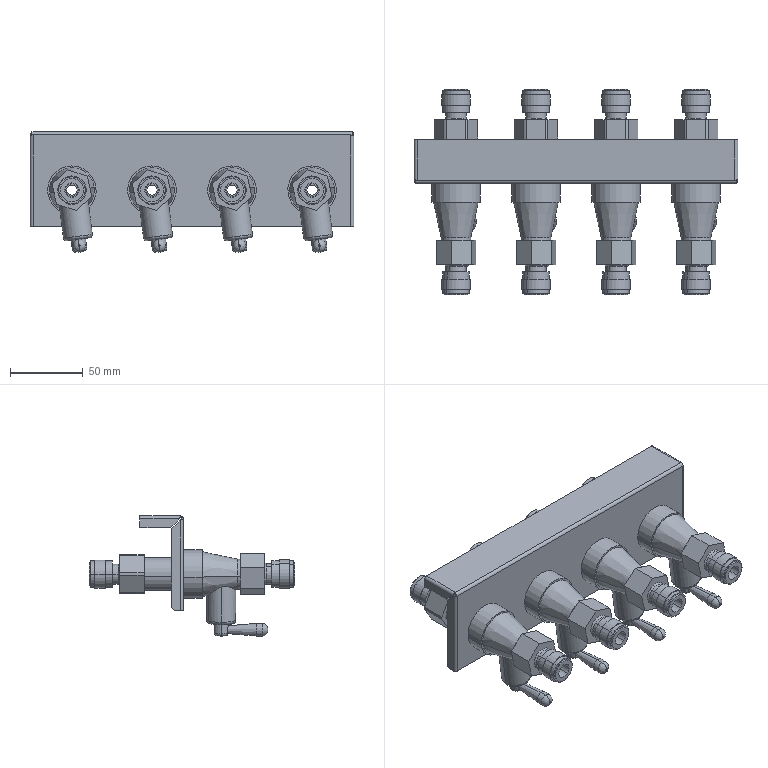Part | SolidWorks | features ReferencePattern 3, AEMSimFeature 1, LocalLPattern 1 | 13 solids | 504 faces | box 222.4 x 141.4 x 82.578 mm | volume 275099 mm3 | cylinder 240 | plane 188 | cone 40 | torus 28 | spline 8 | commonest cylinder face diameters 30 x28 10 x16 14 x16 16 x16 18.2 x16 18.3 x16